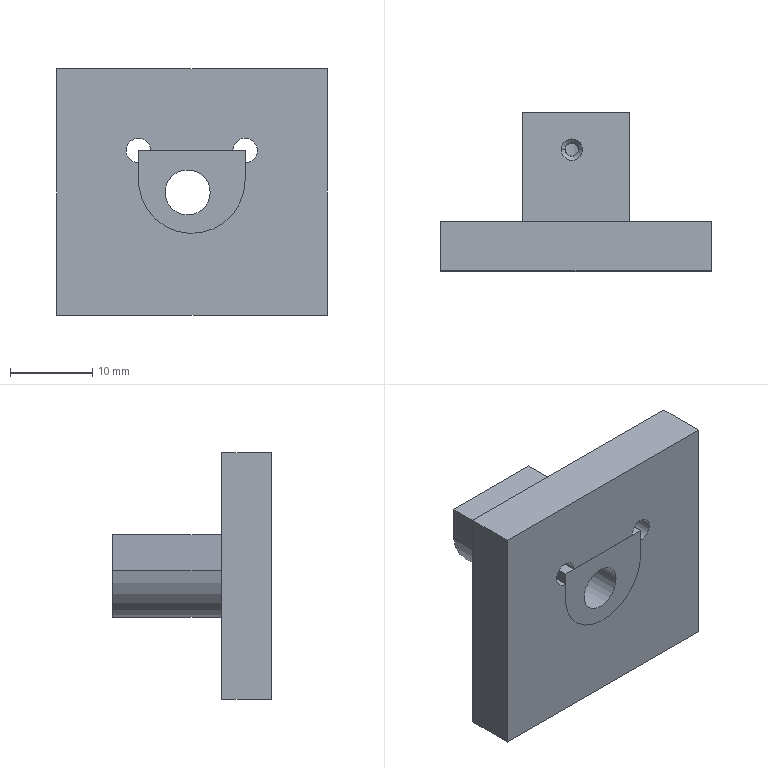NC program | NX | posted with a generic post | part box 32.951 x 19.3 x 30.1 mm
Lines 1 to 1088 of 2936:
N10 G17 G21 G94 G90
(PLANAR_MILL_1 , TOOL : D2)
N12 T02 M6
N14 G54
N16 G17 G0 G90 X0.034 Y0.295 B0. C0. S9500 M3
N18 G43 Z30. H2
N20 Z0.5
N22 G94 G1 X-0.05 Y0.514 Z0.492 F1200.
N24 Y-0.563 Z0.454
N26 X0.058 Y-0.281 Z0.444
N28 Y0.233 Z0.426
N30 X-0.05 Y0.514 Z0.415
N32 Y-0.563 Z0.378
N34 X0.058 Y-0.281 Z0.367
N36 Y0.233 Z0.349
N38 X-0.05 Y0.514 Z0.339
N40 Y-0.563 Z0.301
N42 X0.058 Y-0.281 Z0.29
N44 Y0.233 Z0.272
N46 X-0.05 Y0.514 Z0.262
N48 Y-0.563 Z0.224
N50 X0.058 Y-0.281 Z0.214
N52 Y0.233 Z0.196
N54 X-0.05 Y0.514 Z0.185
N56 Y-0.563 Z0.148
N58 X0.058 Y-0.281 Z0.137
N60 Y0.233 Z0.119
N62 X-0.05 Y0.514 Z0.109
N64 Y-0.563 Z0.071
N66 X0.058 Y-0.281 Z0.061
N68 Y0.233 Z0.043
N70 X-0.05 Y0.514 Z0.032
N72 Y-0.563 Z-0.006
N74 X0.058 Y-0.281 Z-0.016
N76 Y0.233 Z-0.034
N78 X-0.05 Y0.514 Z-0.045
N80 Y-0.563 Z-0.082
N82 X0.058 Y-0.281 Z-0.093
N84 Y0.233 Z-0.111
N86 X-0.05 Y0.514 Z-0.121
N88 Y-0.024 Z-0.14
N90 Y-0.563
N92 G3 X-0.05 Y0.514 R1.5
N94 G1 Y-0.024
N96 X-1.05
N98 Y-2.48
N100 X-0.976 Y-2.479
N102 G3 X-1.05 Y2.443 R2.5
N104 G1 Y-0.024
N106 X-2.05
N108 Y-3.491
N110 X-0.882 Y-3.478
N112 G3 X-1.45 Y3.476 R3.5
N114 G1 X-2.05
N116 Y-0.024
N118 X-3.05
N120 Y-4.502
N122 X-0.799 Y-4.477
N124 G3 X-1.45 Y4.476 R4.5
N126 G1 X-3.05
N128 Y-0.024
N130 X-4.05
N132 Y-5.024
N134 G2 X-5.05 Y-6.024 R1.
N136 G3 X-4.55 Y-6.519 R-0.5
N138 G2 X-3.561 Y-5.508 R1.
N140 G1 X-0.725 Y-5.476
N142 G3 X-1.45 Y5.476 R5.5
N144 G1 X-3.55
N146 G2 X-4.55 Y6.476 R1.
N148 G3 X-5.05 Y5.976 R-0.5
N150 G2 X-4.05 Y4.976 R1.
N152 G1 Y-0.024
N154 Z0.36
N156 G0 X0.034 Y0.295
N158 G1 X-0.05 Y0.514 Z0.352
N160 Y-0.563 Z0.314
N162 X0.058 Y-0.281 Z0.304
N164 Y0.233 Z0.286
N166 X-0.05 Y0.514 Z0.275
N168 Y-0.563 Z0.238
N170 X0.058 Y-0.281 Z0.227
N172 Y0.233 Z0.209
N174 X-0.05 Y0.514 Z0.199
N176 Y-0.563 Z0.161
N178 X0.058 Y-0.281 Z0.15
N180 Y0.233 Z0.132
N182 X-0.05 Y0.514 Z0.122
N184 Y-0.563 Z0.084
N186 X0.058 Y-0.281 Z0.074
N188 Y0.233 Z0.056
N190 X-0.05 Y0.514 Z0.045
N192 Y-0.563 Z0.008
N194 X0.058 Y-0.281 Z-0.003
N196 Y0.233 Z-0.021
N198 X-0.05 Y0.514 Z-0.031
N200 Y-0.563 Z-0.069
N202 X0.058 Y-0.281 Z-0.079
N204 Y0.233 Z-0.097
N206 X-0.05 Y0.514 Z-0.108
N208 Y-0.563 Z-0.146
N210 X0.058 Y-0.281 Z-0.156
N212 Y0.233 Z-0.174
N214 X-0.05 Y0.514 Z-0.185
N216 Y-0.563 Z-0.222
N218 X0.058 Y-0.281 Z-0.233
N220 Y0.233 Z-0.251
N222 X-0.05 Y0.514 Z-0.261
N224 Y-0.024 Z-0.28
N226 Y-0.563
N228 G3 X-0.05 Y0.514 R1.5
N230 G1 Y-0.024
N232 X-1.05
N234 Y-2.48
N236 X-0.976 Y-2.479
N238 G3 X-1.05 Y2.443 R2.5
N240 G1 Y-0.024
N242 X-2.05
N244 Y-3.491
N246 X-0.882 Y-3.478
N248 G3 X-1.45 Y3.476 R3.5
N250 G1 X-2.05
N252 Y-0.024
N254 X-3.05
N256 Y-4.502
N258 X-0.799 Y-4.477
N260 G3 X-1.45 Y4.476 R4.5
N262 G1 X-3.05
N264 Y-0.024
N266 X-4.05
N268 Y-5.024
N270 G2 X-5.05 Y-6.024 R1.
N272 G3 X-4.55 Y-6.519 R-0.5
N274 G2 X-3.561 Y-5.508 R1.
N276 G1 X-0.725 Y-5.476
N278 G3 X-1.45 Y5.476 R5.5
N280 G1 X-3.55
N282 G2 X-4.55 Y6.476 R1.
N284 G3 X-5.05 Y5.976 R-0.5
N286 G2 X-4.05 Y4.976 R1.
N288 G1 Y-0.024
N290 Z0.22
N292 G0 X0.034 Y0.295
N294 G1 X-0.05 Y0.514 Z0.212
N296 Y-0.563 Z0.174
N298 X0.058 Y-0.281 Z0.164
N300 Y0.233 Z0.146
N302 X-0.05 Y0.514 Z0.135
N304 Y-0.563 Z0.098
N306 X0.058 Y-0.281 Z0.087
N308 Y0.233 Z0.069
N310 X-0.05 Y0.514 Z0.059
N312 Y-0.563 Z0.021
N314 X0.058 Y-0.281 Z0.01
N316 Y0.233 Z-0.008
N318 X-0.05 Y0.514 Z-0.018
N320 Y-0.563 Z-0.056
N322 X0.058 Y-0.281 Z-0.066
N324 Y0.233 Z-0.084
N326 X-0.05 Y0.514 Z-0.095
N328 Y-0.563 Z-0.132
N330 X0.058 Y-0.281 Z-0.143
N332 Y0.233 Z-0.161
N334 X-0.05 Y0.514 Z-0.171
N336 Y-0.563 Z-0.209
N338 X0.058 Y-0.281 Z-0.219
N340 Y0.233 Z-0.237
N342 X-0.05 Y0.514 Z-0.248
N344 Y-0.563 Z-0.286
N346 X0.058 Y-0.281 Z-0.296
N348 Y0.233 Z-0.314
N350 X-0.05 Y0.514 Z-0.325
N352 Y-0.563 Z-0.362
N354 X0.058 Y-0.281 Z-0.373
N356 Y0.233 Z-0.391
N358 X-0.05 Y0.514 Z-0.401
N360 Y-0.024 Z-0.42
N362 Y-0.563
N364 G3 X-0.05 Y0.514 R1.5
N366 G1 Y-0.024
N368 X-1.05
N370 Y-2.48
N372 X-0.976 Y-2.479
N374 G3 X-1.05 Y2.443 R2.5
N376 G1 Y-0.024
N378 X-2.05
N380 Y-3.491
N382 X-0.882 Y-3.478
N384 G3 X-1.45 Y3.476 R3.5
N386 G1 X-2.05
N388 Y-0.024
N390 X-3.05
N392 Y-4.502
N394 X-0.799 Y-4.477
N396 G3 X-1.45 Y4.476 R4.5
N398 G1 X-3.05
N400 Y-0.024
N402 X-4.05
N404 Y-5.024
N406 G2 X-5.05 Y-6.024 R1.
N408 G3 X-4.55 Y-6.519 R-0.5
N410 G2 X-3.561 Y-5.508 R1.
N412 G1 X-0.725 Y-5.476
N414 G3 X-1.45 Y5.476 R5.5
N416 G1 X-3.55
N418 G2 X-4.55 Y6.476 R1.
N420 G3 X-5.05 Y5.976 R-0.5
N422 G2 X-4.05 Y4.976 R1.
N424 G1 Y-0.024
N426 Z0.08
N428 G0 X0.034 Y0.295
N430 G1 X-0.05 Y0.514 Z0.072
N432 Y-0.563 Z0.034
N434 X0.058 Y-0.281 Z0.024
N436 Y0.233 Z0.006
N438 X-0.05 Y0.514 Z-0.005
N440 Y-0.563 Z-0.042
N442 X0.058 Y-0.281 Z-0.053
N444 Y0.233 Z-0.071
N446 X-0.05 Y0.514 Z-0.081
N448 Y-0.563 Z-0.119
N450 X0.058 Y-0.281 Z-0.13
N452 Y0.233 Z-0.148
N454 X-0.05 Y0.514 Z-0.158
N456 Y-0.563 Z-0.196
N458 X0.058 Y-0.281 Z-0.206
N460 Y0.233 Z-0.224
N462 X-0.05 Y0.514 Z-0.235
N464 Y-0.563 Z-0.272
N466 X0.058 Y-0.281 Z-0.283
N468 Y0.233 Z-0.301
N470 X-0.05 Y0.514 Z-0.311
N472 Y-0.563 Z-0.349
N474 X0.058 Y-0.281 Z-0.359
N476 Y0.233 Z-0.377
N478 X-0.05 Y0.514 Z-0.388
N480 Y-0.563 Z-0.426
N482 X0.058 Y-0.281 Z-0.436
N484 Y0.233 Z-0.454
N486 X-0.05 Y0.514 Z-0.465
N488 Y-0.563 Z-0.502
N490 X0.058 Y-0.281 Z-0.513
N492 Y0.233 Z-0.531
N494 X-0.05 Y0.514 Z-0.541
N496 Y-0.024 Z-0.56
N498 Y-0.563
N500 G3 X-0.05 Y0.514 R1.5
N502 G1 Y-0.024
N504 X-1.05
N506 Y-2.48
N508 X-0.976 Y-2.479
N510 G3 X-1.05 Y2.443 R2.5
N512 G1 Y-0.024
N514 X-2.05
N516 Y-3.491
N518 X-0.882 Y-3.478
N520 G3 X-1.45 Y3.476 R3.5
N522 G1 X-2.05
N524 Y-0.024
N526 X-3.05
N528 Y-4.502
N530 X-0.799 Y-4.477
N532 G3 X-1.45 Y4.476 R4.5
N534 G1 X-3.05
N536 Y-0.024
N538 X-4.05
N540 Y-5.024
N542 G2 X-5.05 Y-6.024 R1.
N544 G3 X-4.55 Y-6.519 R-0.5
N546 G2 X-3.561 Y-5.508 R1.
N548 G1 X-0.725 Y-5.476
N550 G3 X-1.45 Y5.476 R5.5
N552 G1 X-3.55
N554 G2 X-4.55 Y6.476 R1.
N556 G3 X-5.05 Y5.976 R-0.5
N558 G2 X-4.05 Y4.976 R1.
N560 G1 Y-0.024
N562 Z-0.06
N564 G0 X0.034 Y0.295
N566 G1 X-0.05 Y0.514 Z-0.068
N568 Y-0.563 Z-0.106
N570 X0.058 Y-0.281 Z-0.116
N572 Y0.233 Z-0.134
N574 X-0.05 Y0.514 Z-0.145
N576 Y-0.563 Z-0.182
N578 X0.058 Y-0.281 Z-0.193
N580 Y0.233 Z-0.211
N582 X-0.05 Y0.514 Z-0.221
N584 Y-0.563 Z-0.259
N586 X0.058 Y-0.281 Z-0.27
N588 Y0.233 Z-0.288
N590 X-0.05 Y0.514 Z-0.298
N592 Y-0.563 Z-0.336
N594 X0.058 Y-0.281 Z-0.346
N596 Y0.233 Z-0.364
N598 X-0.05 Y0.514 Z-0.375
N600 Y-0.563 Z-0.412
N602 X0.058 Y-0.281 Z-0.423
N604 Y0.233 Z-0.441
N606 X-0.05 Y0.514 Z-0.451
N608 Y-0.563 Z-0.489
N610 X0.058 Y-0.281 Z-0.499
N612 Y0.233 Z-0.517
N614 X-0.05 Y0.514 Z-0.528
N616 Y-0.563 Z-0.566
N618 X0.058 Y-0.281 Z-0.576
N620 Y0.233 Z-0.594
N622 X-0.05 Y0.514 Z-0.605
N624 Y-0.563 Z-0.642
N626 X0.058 Y-0.281 Z-0.653
N628 Y0.233 Z-0.671
N630 X-0.05 Y0.514 Z-0.681
N632 Y-0.024 Z-0.7
N634 Y-0.563
N636 G3 X-0.05 Y0.514 R1.5
N638 G1 Y-0.024
N640 X-1.05
N642 Y-2.48
N644 X-0.976 Y-2.479
N646 G3 X-1.05 Y2.443 R2.5
N648 G1 Y-0.024
N650 X-2.05
N652 Y-3.491
N654 X-0.882 Y-3.478
N656 G3 X-1.45 Y3.476 R3.5
N658 G1 X-2.05
N660 Y-0.024
N662 X-3.05
N664 Y-4.502
N666 X-0.799 Y-4.477
N668 G3 X-1.45 Y4.476 R4.5
N670 G1 X-3.05
N672 Y-0.024
N674 X-4.05
N676 Y-5.024
N678 G2 X-5.05 Y-6.024 R1.
N680 G3 X-4.55 Y-6.519 R-0.5
N682 G2 X-3.561 Y-5.508 R1.
N684 G1 X-0.725 Y-5.476
N686 G3 X-1.45 Y5.476 R5.5
N688 G1 X-3.55
N690 G2 X-4.55 Y6.476 R1.
N692 G3 X-5.05 Y5.976 R-0.5
N694 G2 X-4.05 Y4.976 R1.
N696 G1 Y-0.024
N698 Z-0.2
N700 G0 X0.034 Y0.295
N702 G1 X-0.05 Y0.514 Z-0.208
N704 Y-0.563 Z-0.246
N706 X0.058 Y-0.281 Z-0.256
N708 Y0.233 Z-0.274
N710 X-0.05 Y0.514 Z-0.285
N712 Y-0.563 Z-0.322
N714 X0.058 Y-0.281 Z-0.333
N716 Y0.233 Z-0.351
N718 X-0.05 Y0.514 Z-0.361
N720 Y-0.563 Z-0.399
N722 X0.058 Y-0.281 Z-0.41
N724 Y0.233 Z-0.428
N726 X-0.05 Y0.514 Z-0.438
N728 Y-0.563 Z-0.476
N730 X0.058 Y-0.281 Z-0.486
N732 Y0.233 Z-0.504
N734 X-0.05 Y0.514 Z-0.515
N736 Y-0.563 Z-0.552
N738 X0.058 Y-0.281 Z-0.563
N740 Y0.233 Z-0.581
N742 X-0.05 Y0.514 Z-0.591
N744 Y-0.563 Z-0.629
N746 X0.058 Y-0.281 Z-0.639
N748 Y0.233 Z-0.657
N750 X-0.05 Y0.514 Z-0.668
N752 Y-0.563 Z-0.706
N754 X0.058 Y-0.281 Z-0.716
N756 Y0.233 Z-0.734
N758 X-0.05 Y0.514 Z-0.745
N760 Y-0.563 Z-0.782
N762 X0.058 Y-0.281 Z-0.793
N764 Y0.233 Z-0.811
N766 X-0.05 Y0.514 Z-0.821
N768 Y-0.024 Z-0.84
N770 Y-0.563
N772 G3 X-0.05 Y0.514 R1.5
N774 G1 Y-0.024
N776 X-1.05
N778 Y-2.48
N780 X-0.976 Y-2.479
N782 G3 X-1.05 Y2.443 R2.5
N784 G1 Y-0.024
N786 X-2.05
N788 Y-3.491
N790 X-0.882 Y-3.478
N792 G3 X-1.45 Y3.476 R3.5
N794 G1 X-2.05
N796 Y-0.024
N798 X-3.05
N800 Y-4.502
N802 X-0.799 Y-4.477
N804 G3 X-1.45 Y4.476 R4.5
N806 G1 X-3.05
N808 Y-0.024
N810 X-4.05
N812 Y-5.024
N814 G2 X-5.05 Y-6.024 R1.
N816 G3 X-4.55 Y-6.519 R-0.5
N818 G2 X-3.561 Y-5.508 R1.
N820 G1 X-0.725 Y-5.476
N822 G3 X-1.45 Y5.476 R5.5
N824 G1 X-3.55
N826 G2 X-4.55 Y6.476 R1.
N828 G3 X-5.05 Y5.976 R-0.5
N830 G2 X-4.05 Y4.976 R1.
N832 G1 Y-0.024
N834 Z-0.34
N836 G0 X0.034 Y0.295
N838 G1 X-0.05 Y0.514 Z-0.348
N840 Y-0.563 Z-0.386
N842 X0.058 Y-0.281 Z-0.396
N844 Y0.233 Z-0.414
N846 X-0.05 Y0.514 Z-0.425
N848 Y-0.563 Z-0.462
N850 X0.058 Y-0.281 Z-0.473
N852 Y0.233 Z-0.491
N854 X-0.05 Y0.514 Z-0.501
N856 Y-0.563 Z-0.539
N858 X0.058 Y-0.281 Z-0.55
N860 Y0.233 Z-0.568
N862 X-0.05 Y0.514 Z-0.578
N864 Y-0.563 Z-0.616
N866 X0.058 Y-0.281 Z-0.626
N868 Y0.233 Z-0.644
N870 X-0.05 Y0.514 Z-0.655
N872 Y-0.563 Z-0.692
N874 X0.058 Y-0.281 Z-0.703
N876 Y0.233 Z-0.721
N878 X-0.05 Y0.514 Z-0.731
N880 Y-0.563 Z-0.769
N882 X0.058 Y-0.281 Z-0.779
N884 Y0.233 Z-0.797
N886 X-0.05 Y0.514 Z-0.808
N888 Y-0.563 Z-0.846
N890 X0.058 Y-0.281 Z-0.856
N892 Y0.233 Z-0.874
N894 X-0.05 Y0.514 Z-0.885
N896 Y-0.563 Z-0.922
N898 X0.058 Y-0.281 Z-0.933
N900 Y0.233 Z-0.951
N902 X-0.05 Y0.514 Z-0.961
N904 Y-0.024 Z-0.98
N906 Y-0.563
N908 G3 X-0.05 Y0.514 R1.5
N910 G1 Y-0.024
N912 X-1.05
N914 Y-2.48
N916 X-0.976 Y-2.479
N918 G3 X-1.05 Y2.443 R2.5
N920 G1 Y-0.024
N922 X-2.05
N924 Y-3.491
N926 X-0.882 Y-3.478
N928 G3 X-1.45 Y3.476 R3.5
N930 G1 X-2.05
N932 Y-0.024
N934 X-3.05
N936 Y-4.502
N938 X-0.799 Y-4.477
N940 G3 X-1.45 Y4.476 R4.5
N942 G1 X-3.05
N944 Y-0.024
N946 X-4.05
N948 Y-5.024
N950 G2 X-5.05 Y-6.024 R1.
N952 G3 X-4.55 Y-6.519 R-0.5
N954 G2 X-3.561 Y-5.508 R1.
N956 G1 X-0.725 Y-5.476
N958 G3 X-1.45 Y5.476 R5.5
N960 G1 X-3.55
N962 G2 X-4.55 Y6.476 R1.
N964 G3 X-5.05 Y5.976 R-0.5
N966 G2 X-4.05 Y4.976 R1.
N968 G1 Y-0.024
N970 Z-0.48
N972 G0 X0.034 Y0.295
N974 G1 X-0.05 Y0.514 Z-0.488
N976 Y-0.563 Z-0.526
N978 X0.058 Y-0.281 Z-0.536
N980 Y0.233 Z-0.554
N982 X-0.05 Y0.514 Z-0.565
N984 Y-0.563 Z-0.602
N986 X0.058 Y-0.281 Z-0.613
N988 Y0.233 Z-0.631
N990 X-0.05 Y0.514 Z-0.641
N992 Y-0.563 Z-0.679
N994 X0.058 Y-0.281 Z-0.69
N996 Y0.233 Z-0.708
N998 X-0.05 Y0.514 Z-0.718
N1000 Y-0.563 Z-0.756
N1002 X0.058 Y-0.281 Z-0.766
N1004 Y0.233 Z-0.784
N1006 X-0.05 Y0.514 Z-0.795
N1008 Y-0.563 Z-0.832
N1010 X0.058 Y-0.281 Z-0.843
N1012 Y0.233 Z-0.861
N1014 X-0.05 Y0.514 Z-0.871
N1016 Y-0.563 Z-0.909
N1018 X0.058 Y-0.281 Z-0.919
N1020 Y0.233 Z-0.937
N1022 X-0.05 Y0.514 Z-0.948
N1024 Y-0.563 Z-0.986
N1026 X0.058 Y-0.281 Z-0.996
N1028 Y0.233 Z-1.014
N1030 X-0.05 Y0.514 Z-1.025
N1032 Y-0.563 Z-1.062
N1034 X0.058 Y-0.281 Z-1.073
N1036 Y0.233 Z-1.091
N1038 X-0.05 Y0.514 Z-1.101
N1040 Y-0.024 Z-1.12
N1042 Y-0.563
N1044 G3 X-0.05 Y0.514 R1.5
N1046 G1 Y-0.024
N1048 X-1.05
N1050 Y-2.48
N1052 X-0.976 Y-2.479
N1054 G3 X-1.05 Y2.443 R2.5
N1056 G1 Y-0.024
N1058 X-2.05
N1060 Y-3.491
N1062 X-0.882 Y-3.478
N1064 G3 X-1.45 Y3.476 R3.5
N1066 G1 X-2.05
N1068 Y-0.024
N1070 X-3.05
N1072 Y-4.502
N1074 X-0.799 Y-4.477
N1076 G3 X-1.45 Y4.476 R4.5
N1078 G1 X-3.05
N1080 Y-0.024
N1082 X-4.05
N1084 Y-5.024
N1086 G2 X-5.05 Y-6.024 R1.
N1088 G3 X-4.55 Y-6.519 R-0.5
N1090 G2 X-3.561 Y-5.508 R1.
N1092 G1 X-0.725 Y-5.476
N1094 G3 X-1.45 Y5.476 R5.5
N1096 G1 X-3.55
N1098 G2 X-4.55 Y6.476 R1.
N1100 G3 X-5.05 Y5.976 R-0.5
N1102 G2 X-4.05 Y4.976 R1.
N1104 G1 Y-0.024
N1106 Z-0.62
N1108 G0 X0.034 Y0.295
N1110 G1 X-0.05 Y0.514 Z-0.628
N1112 Y-0.563 Z-0.666
N1114 X0.058 Y-0.281 Z-0.676
N1116 Y0.233 Z-0.694
N1118 X-0.05 Y0.514 Z-0.705
N1120 Y-0.563 Z-0.742
N1122 X0.058 Y-0.281 Z-0.753
N1124 Y0.233 Z-0.771
N1126 X-0.05 Y0.514 Z-0.781
N1128 Y-0.563 Z-0.819
N1130 X0.058 Y-0.281 Z-0.83
N1132 Y0.233 Z-0.848
N1134 X-0.05 Y0.514 Z-0.858
N1136 Y-0.563 Z-0.896
N1138 X0.058 Y-0.281 Z-0.906
N1140 Y0.233 Z-0.924
N1142 X-0.05 Y0.514 Z-0.935
N1144 Y-0.563 Z-0.972
N1146 X0.058 Y-0.281 Z-0.983
N1148 Y0.233 Z-1.001
N1150 X-0.05 Y0.514 Z-1.011
N1152 Y-0.563 Z-1.049
N1154 X0.058 Y-0.281 Z-1.059
N1156 Y0.233 Z-1.077
N1158 X-0.05 Y0.514 Z-1.088
N1160 Y-0.563 Z-1.126
N1162 X0.058 Y-0.281 Z-1.136
N1164 Y0.233 Z-1.154
N1166 X-0.05 Y0.514 Z-1.165
N1168 Y-0.563 Z-1.202
N1170 X0.058 Y-0.281 Z-1.213
N1172 Y0.233 Z-1.231
N1174 X-0.05 Y0.514 Z-1.241
N1176 Y-0.024 Z-1.26
N1178 Y-0.563
N1180 G3 X-0.05 Y0.514 R1.5
N1182 G1 Y-0.024
N1184 X-1.05
N1186 Y-2.48
N1188 X-0.976 Y-2.479
N1190 G3 X-1.05 Y2.443 R2.5
N1192 G1 Y-0.024
N1194 X-2.05
N1196 Y-3.491
N1198 X-0.882 Y-3.478
N1200 G3 X-1.45 Y3.476 R3.5
N1202 G1 X-2.05
N1204 Y-0.024
N1206 X-3.05
N1208 Y-4.502
N1210 X-0.799 Y-4.477
N1212 G3 X-1.45 Y4.476 R4.5
N1214 G1 X-3.05
N1216 Y-0.024
N1218 X-4.05
N1220 Y-5.024
N1222 G2 X-5.05 Y-6.024 R1.
N1224 G3 X-4.55 Y-6.519 R-0.5
N1226 G2 X-3.561 Y-5.508 R1.
N1228 G1 X-0.725 Y-5.476
N1230 G3 X-1.45 Y5.476 R5.5
N1232 G1 X-3.55
N1234 G2 X-4.55 Y6.476 R1.
N1236 G3 X-5.05 Y5.976 R-0.5
N1238 G2 X-4.05 Y4.976 R1.
N1240 G1 Y-0.024
N1242 Z-0.76
N1244 G0 X0.034 Y0.295
N1246 G1 X-0.05 Y0.514 Z-0.768
N1248 Y-0.563 Z-0.806
N1250 X0.058 Y-0.281 Z-0.816
N1252 Y0.233 Z-0.834
N1254 X-0.05 Y0.514 Z-0.845
N1256 Y-0.563 Z-0.882
N1258 X0.058 Y-0.281 Z-0.893
N1260 Y0.233 Z-0.911
N1262 X-0.05 Y0.514 Z-0.921
N1264 Y-0.563 Z-0.959
N1266 X0.058 Y-0.281 Z-0.97
N1268 Y0.233 Z-0.988
N1270 X-0.05 Y0.514 Z-0.998
N1272 Y-0.563 Z-1.036
N1274 X0.058 Y-0.281 Z-1.046
N1276 Y0.233 Z-1.064
N1278 X-0.05 Y0.514 Z-1.075
N1280 Y-0.563 Z-1.112
N1282 X0.058 Y-0.281 Z-1.123
N1284 Y0.233 Z-1.141
N1286 X-0.05 Y0.514 Z-1.151
N1288 Y-0.563 Z-1.189
N1290 X0.058 Y-0.281 Z-1.199
N1292 Y0.233 Z-1.217
N1294 X-0.05 Y0.514 Z-1.228
N1296 Y-0.563 Z-1.266
N1298 X0.058 Y-0.281 Z-1.276
N1300 Y0.233 Z-1.294
N1302 X-0.05 Y0.514 Z-1.305
N1304 Y-0.563 Z-1.342
N1306 X0.058 Y-0.281 Z-1.353
N1308 Y0.233 Z-1.371
N1310 X-0.05 Y0.514 Z-1.381
N1312 Y-0.024 Z-1.4
N1314 Y-0.563
N1316 G3 X-0.05 Y0.514 R1.5
N1318 G1 Y-0.024
N1320 X-1.05
N1322 Y-2.48
N1324 X-0.976 Y-2.479
N1326 G3 X-1.05 Y2.443 R2.5
N1328 G1 Y-0.024
N1330 X-2.05
N1332 Y-3.491
N1334 X-0.882 Y-3.478
N1336 G3 X-1.45 Y3.476 R3.5
N1338 G1 X-2.05
N1340 Y-0.024
N1342 X-3.05
N1344 Y-4.502
N1346 X-0.799 Y-4.477
N1348 G3 X-1.45 Y4.476 R4.5
N1350 G1 X-3.05
N1352 Y-0.024
N1354 X-4.05
N1356 Y-5.024
N1358 G2 X-5.05 Y-6.024 R1.
N1360 G3 X-4.55 Y-6.519 R-0.5
N1362 G2 X-3.561 Y-5.508 R1.
N1364 G1 X-0.725 Y-5.476
N1366 G3 X-1.45 Y5.476 R5.5
N1368 G1 X-3.55
N1370 G2 X-4.55 Y6.476 R1.
N1372 G3 X-5.05 Y5.976 R-0.5
N1374 G2 X-4.05 Y4.976 R1.
N1376 G1 Y-0.024
N1378 Z-0.9
N1380 G0 X0.034 Y0.295
N1382 G1 X-0.05 Y0.514 Z-0.908
N1384 Y-0.563 Z-0.946
N1386 X0.058 Y-0.281 Z-0.956
N1388 Y0.233 Z-0.974
N1390 X-0.05 Y0.514 Z-0.985
N1392 Y-0.563 Z-1.022
N1394 X0.058 Y-0.281 Z-1.033
N1396 Y0.233 Z-1.051
N1398 X-0.05 Y0.514 Z-1.061
N1400 Y-0.563 Z-1.099
N1402 X0.058 Y-0.281 Z-1.11
N1404 Y0.233 Z-1.128
N1406 X-0.05 Y0.514 Z-1.138
N1408 Y-0.563 Z-1.176
N1410 X0.058 Y-0.281 Z-1.186
N1412 Y0.233 Z-1.204
N1414 X-0.05 Y0.514 Z-1.215
N1416 Y-0.563 Z-1.252
N1418 X0.058 Y-0.281 Z-1.263
N1420 Y0.233 Z-1.281
N1422 X-0.05 Y0.514 Z-1.291
N1424 Y-0.563 Z-1.329
N1426 X0.058 Y-0.281 Z-1.339
N1428 Y0.233 Z-1.357
N1430 X-0.05 Y0.514 Z-1.368
N1432 Y-0.563 Z-1.406
N1434 X0.058 Y-0.281 Z-1.416
N1436 Y0.233 Z-1.434
N1438 X-0.05 Y0.514 Z-1.445
N1440 Y-0.563 Z-1.482
N1442 X0.058 Y-0.281 Z-1.493
N1444 Y0.233 Z-1.511
N1446 X-0.05 Y0.514 Z-1.521
N1448 Y-0.024 Z-1.54
N1450 Y-0.563
N1452 G3 X-0.05 Y0.514 R1.5
N1454 G1 Y-0.024
N1456 X-1.05
N1458 Y-2.48
N1460 X-0.976 Y-2.479
N1462 G3 X-1.05 Y2.443 R2.5
N1464 G1 Y-0.024
N1466 X-2.05
N1468 Y-3.491
N1470 X-0.882 Y-3.478
N1472 G3 X-1.45 Y3.476 R3.5
N1474 G1 X-2.05
N1476 Y-0.024
N1478 X-3.05
N1480 Y-4.502
N1482 X-0.799 Y-4.477
N1484 G3 X-1.45 Y4.476 R4.5
N1486 G1 X-3.05
N1488 Y-0.024
N1490 X-4.05
N1492 Y-5.024
N1494 G2 X-5.05 Y-6.024 R1.
N1496 G3 X-4.55 Y-6.519 R-0.5
N1498 G2 X-3.561 Y-5.508 R1.
N1500 G1 X-0.725 Y-5.476
N1502 G3 X-1.45 Y5.476 R5.5
N1504 G1 X-3.55
N1506 G2 X-4.55 Y6.476 R1.
N1508 G3 X-5.05 Y5.976 R-0.5
N1510 G2 X-4.05 Y4.976 R1.
N1512 G1 Y-0.024
N1514 Z-1.04
N1516 G0 X0.034 Y0.295
N1518 G1 X-0.05 Y0.514 Z-1.048
N1520 Y-0.563 Z-1.086
N1522 X0.058 Y-0.281 Z-1.096
N1524 Y0.233 Z-1.114
N1526 X-0.05 Y0.514 Z-1.125
N1528 Y-0.563 Z-1.162
N1530 X0.058 Y-0.281 Z-1.173
N1532 Y0.233 Z-1.191
N1534 X-0.05 Y0.514 Z-1.201
N1536 Y-0.563 Z-1.239
N1538 X0.058 Y-0.281 Z-1.25
N1540 Y0.233 Z-1.268
N1542 X-0.05 Y0.514 Z-1.278
N1544 Y-0.563 Z-1.316
N1546 X0.058 Y-0.281 Z-1.326
N1548 Y0.233 Z-1.344
N1550 X-0.05 Y0.514 Z-1.355
N1552 Y-0.563 Z-1.392
N1554 X0.058 Y-0.281 Z-1.403
N1556 Y0.233 Z-1.421
N1558 X-0.05 Y0.514 Z-1.431
N1560 Y-0.563 Z-1.469
N1562 X0.058 Y-0.281 Z-1.479
N1564 Y0.233 Z-1.497
N1566 X-0.05 Y0.514 Z-1.508
N1568 Y-0.563 Z-1.546
N1570 X0.058 Y-0.281 Z-1.556
N1572 Y0.233 Z-1.574
N1574 X-0.05 Y0.514 Z-1.585
N1576 Y-0.563 Z-1.622
N1578 X0.058 Y-0.281 Z-1.633
N1580 Y0.233 Z-1.651
N1582 X-0.05 Y0.514 Z-1.661
N1584 Y-0.024 Z-1.68
N1586 Y-0.563
N1588 G3 X-0.05 Y0.514 R1.5
N1590 G1 Y-0.024
N1592 X-1.05
N1594 Y-2.48
N1596 X-0.976 Y-2.479
N1598 G3 X-1.05 Y2.443 R2.5
N1600 G1 Y-0.024
N1602 X-2.05
N1604 Y-3.491
N1606 X-0.882 Y-3.478
N1608 G3 X-1.45 Y3.476 R3.5
N1610 G1 X-2.05
N1612 Y-0.024
N1614 X-3.05
N1616 Y-4.502
N1618 X-0.799 Y-4.477
N1620 G3 X-1.45 Y4.476 R4.5
N1622 G1 X-3.05
N1624 Y-0.024
N1626 X-4.05
N1628 Y-5.024
N1630 G2 X-5.05 Y-6.024 R1.
N1632 G3 X-4.55 Y-6.519 R-0.5
N1634 G2 X-3.561 Y-5.508 R1.
N1636 G1 X-0.725 Y-5.476
N1638 G3 X-1.45 Y5.476 R5.5
N1640 G1 X-3.55
N1642 G2 X-4.55 Y6.476 R1.
N1644 G3 X-5.05 Y5.976 R-0.5
N1646 G2 X-4.05 Y4.976 R1.
N1648 G1 Y-0.024
N1650 Z-1.18
N1652 G0 X0.034 Y0.295
N1654 G1 X-0.05 Y0.514 Z-1.188
N1656 Y-0.563 Z-1.226
N1658 X0.058 Y-0.281 Z-1.236
N1660 Y0.233 Z-1.254
N1662 X-0.05 Y0.514 Z-1.265
N1664 Y-0.563 Z-1.302
N1666 X0.058 Y-0.281 Z-1.313
N1668 Y0.233 Z-1.331
N1670 X-0.05 Y0.514 Z-1.341
N1672 Y-0.563 Z-1.379
N1674 X0.058 Y-0.281 Z-1.39
N1676 Y0.233 Z-1.408
N1678 X-0.05 Y0.514 Z-1.418
N1680 Y-0.563 Z-1.456
N1682 X0.058 Y-0.281 Z-1.466
N1684 Y0.233 Z-1.484
N1686 X-0.05 Y0.514 Z-1.495
N1688 Y-0.563 Z-1.532
N1690 X0.058 Y-0.281 Z-1.543
N1692 Y0.233 Z-1.561
N1694 X-0.05 Y0.514 Z-1.571
N1696 Y-0.563 Z-1.609
N1698 X0.058 Y-0.281 Z-1.619
N1700 Y0.233 Z-1.637
N1702 X-0.05 Y0.514 Z-1.648
N1704 Y-0.563 Z-1.686
N1706 X0.058 Y-0.281 Z-1.696
N1708 Y0.233 Z-1.714
N1710 X-0.05 Y0.514 Z-1.725
N1712 Y-0.563 Z-1.762
N1714 X0.058 Y-0.281 Z-1.773
N1716 Y0.233 Z-1.791
N1718 X-0.05 Y0.514 Z-1.801
N1720 Y-0.024 Z-1.82
N1722 Y-0.563
N1724 G3 X-0.05 Y0.514 R1.5
N1726 G1 Y-0.024
N1728 X-1.05
N1730 Y-2.48
N1732 X-0.976 Y-2.479
N1734 G3 X-1.05 Y2.443 R2.5
N1736 G1 Y-0.024
N1738 X-2.05
N1740 Y-3.491
N1742 X-0.882 Y-3.478
N1744 G3 X-1.45 Y3.476 R3.5
N1746 G1 X-2.05
N1748 Y-0.024
N1750 X-3.05
N1752 Y-4.502
N1754 X-0.799 Y-4.477
N1756 G3 X-1.45 Y4.476 R4.5
N1758 G1 X-3.05
N1760 Y-0.024
N1762 X-4.05
N1764 Y-5.024
N1766 G2 X-5.05 Y-6.024 R1.
N1768 G3 X-4.55 Y-6.519 R-0.5
N1770 G2 X-3.561 Y-5.508 R1.
N1772 G1 X-0.725 Y-5.476
N1774 G3 X-1.45 Y5.476 R5.5
N1776 G1 X-3.55
N1778 G2 X-4.55 Y6.476 R1.
N1780 G3 X-5.05 Y5.976 R-0.5
N1782 G2 X-4.05 Y4.976 R1.
N1784 G1 Y-0.024
N1786 Z-1.32
N1788 G0 X0.034 Y0.295
N1790 G1 X-0.05 Y0.514 Z-1.328
N1792 Y-0.563 Z-1.366
N1794 X0.058 Y-0.281 Z-1.376
N1796 Y0.233 Z-1.394
N1798 X-0.05 Y0.514 Z-1.405
N1800 Y-0.563 Z-1.442
N1802 X0.058 Y-0.281 Z-1.453
N1804 Y0.233 Z-1.471
N1806 X-0.05 Y0.514 Z-1.481
N1808 Y-0.563 Z-1.519
N1810 X0.058 Y-0.281 Z-1.53
N1812 Y0.233 Z-1.548
N1814 X-0.05 Y0.514 Z-1.558
N1816 Y-0.563 Z-1.596
N1818 X0.058 Y-0.281 Z-1.606
N1820 Y0.233 Z-1.624
N1822 X-0.05 Y0.514 Z-1.635
N1824 Y-0.563 Z-1.672
N1826 X0.058 Y-0.281 Z-1.683
N1828 Y0.233 Z-1.701
N1830 X-0.05 Y0.514 Z-1.711
N1832 Y-0.563 Z-1.749
N1834 X0.058 Y-0.281 Z-1.759
N1836 Y0.233 Z-1.777
N1838 X-0.05 Y0.514 Z-1.788
N1840 Y-0.563 Z-1.826
N1842 X0.058 Y-0.281 Z-1.836
N1844 Y0.233 Z-1.854
N1846 X-0.05 Y0.514 Z-1.865
N1848 Y-0.563 Z-1.902
N1850 X0.058 Y-0.281 Z-1.913
N1852 Y0.233 Z-1.931
N1854 X-0.05 Y0.514 Z-1.941
N1856 Y-0.024 Z-1.96
N1858 Y-0.563
N1860 G3 X-0.05 Y0.514 R1.5
N1862 G1 Y-0.024
N1864 X-1.05
N1866 Y-2.48
N1868 X-0.976 Y-2.479
N1870 G3 X-1.05 Y2.443 R2.5
N1872 G1 Y-0.024
N1874 X-2.05
N1876 Y-3.491
N1878 X-0.882 Y-3.478
N1880 G3 X-1.45 Y3.476 R3.5
N1882 G1 X-2.05
N1884 Y-0.024
N1886 X-3.05
N1888 Y-4.502
N1890 X-0.799 Y-4.477
N1892 G3 X-1.45 Y4.476 R4.5
N1894 G1 X-3.05
N1896 Y-0.024
N1898 X-4.05
N1900 Y-5.024
N1902 G2 X-5.05 Y-6.024 R1.
N1904 G3 X-4.55 Y-6.519 R-0.5
N1906 G2 X-3.561 Y-5.508 R1.
N1908 G1 X-0.725 Y-5.476
N1910 G3 X-1.45 Y5.476 R5.5
N1912 G1 X-3.55
N1914 G2 X-4.55 Y6.476 R1.
N1916 G3 X-5.05 Y5.976 R-0.5
N1918 G2 X-4.05 Y4.976 R1.
N1920 G1 Y-0.024
N1922 Z-1.46
N1924 G0 X0.034 Y0.295
N1926 G1 X-0.05 Y0.514 Z-1.468
N1928 Y-0.563 Z-1.506
N1930 X0.058 Y-0.281 Z-1.516
N1932 Y0.233 Z-1.534
N1934 X-0.05 Y0.514 Z-1.545
N1936 Y-0.563 Z-1.582
N1938 X0.058 Y-0.281 Z-1.593
N1940 Y0.233 Z-1.611
N1942 X-0.05 Y0.514 Z-1.621
N1944 Y-0.563 Z-1.659
N1946 X0.058 Y-0.281 Z-1.67
N1948 Y0.233 Z-1.688
N1950 X-0.05 Y0.514 Z-1.698
N1952 Y-0.563 Z-1.736
N1954 X0.058 Y-0.281 Z-1.746
N1956 Y0.233 Z-1.764
N1958 X-0.05 Y0.514 Z-1.775
N1960 Y-0.563 Z-1.812
N1962 X0.058 Y-0.281 Z-1.823
N1964 Y0.233 Z-1.841
N1966 X-0.05 Y0.514 Z-1.851
N1968 Y-0.563 Z-1.889
N1970 X0.058 Y-0.281 Z-1.899
N1972 Y0.233 Z-1.917
N1974 X-0.05 Y0.514 Z-1.928
N1976 Y-0.563 Z-1.966
N1978 X0.058 Y-0.281 Z-1.976
N1980 Y0.233 Z-1.994
N1982 X-0.05 Y0.514 Z-2.005
N1984 Y-0.563 Z-2.042
N1986 X0.058 Y-0.281 Z-2.053
N1988 Y0.233 Z-2.071
N1990 X-0.05 Y0.514 Z-2.081
N1992 Y-0.024 Z-2.1
N1994 Y-0.563
N1996 G3 X-0.05 Y0.514 R1.5
N1998 G1 Y-0.024
N2000 X-1.05
N2002 Y-2.48
N2004 X-0.976 Y-2.479
N2006 G3 X-1.05 Y2.443 R2.5
N2008 G1 Y-0.024
N2010 X-2.05
N2012 Y-3.491
N2014 X-0.882 Y-3.478
N2016 G3 X-1.45 Y3.476 R3.5
N2018 G1 X-2.05
N2020 Y-0.024
N2022 X-3.05
N2024 Y-4.502
N2026 X-0.799 Y-4.477
N2028 G3 X-1.45 Y4.476 R4.5
N2030 G1 X-3.05
N2032 Y-0.024
N2034 X-4.05
N2036 Y-5.024
N2038 G2 X-5.05 Y-6.024 R1.
N2040 G3 X-4.55 Y-6.519 R-0.5
N2042 G2 X-3.561 Y-5.508 R1.
N2044 G1 X-0.725 Y-5.476
N2046 G3 X-1.45 Y5.476 R5.5
N2048 G1 X-3.55
N2050 G2 X-4.55 Y6.476 R1.
N2052 G3 X-5.05 Y5.976 R-0.5
N2054 G2 X-4.05 Y4.976 R1.
N2056 G1 Y-0.024
N2058 Z-1.6
N2060 G0 X0.034 Y0.295
N2062 G1 X-0.05 Y0.514 Z-1.608
N2064 Y-0.563 Z-1.646
N2066 X0.058 Y-0.281 Z-1.656
N2068 Y0.233 Z-1.674
N2070 X-0.05 Y0.514 Z-1.685
N2072 Y-0.563 Z-1.722
N2074 X0.058 Y-0.281 Z-1.733
N2076 Y0.233 Z-1.751
N2078 X-0.05 Y0.514 Z-1.761
N2080 Y-0.563 Z-1.799
N2082 X0.058 Y-0.281 Z-1.81
N2084 Y0.233 Z-1.828
N2086 X-0.05 Y0.514 Z-1.838
N2088 Y-0.563 Z-1.876
N2090 X0.058 Y-0.281 Z-1.886
N2092 Y0.233 Z-1.904
N2094 X-0.05 Y0.514 Z-1.915
N2096 Y-0.563 Z-1.952
N2098 X0.058 Y-0.281 Z-1.963
N2100 Y0.233 Z-1.981
N2102 X-0.05 Y0.514 Z-1.991
N2104 Y-0.563 Z-2.029
N2106 X0.058 Y-0.281 Z-2.039
N2108 Y0.233 Z-2.057
N2110 X-0.05 Y0.514 Z-2.068
N2112 Y-0.563 Z-2.106
N2114 X0.058 Y-0.281 Z-2.116
N2116 Y0.233 Z-2.134
N2118 X-0.05 Y0.514 Z-2.145
N2120 Y-0.563 Z-2.182
N2122 X0.058 Y-0.281 Z-2.193
N2124 Y0.233 Z-2.211
N2126 X-0.05 Y0.514 Z-2.221
N2128 Y-0.024 Z-2.24
N2130 Y-0.563
N2132 G3 X-0.05 Y0.514 R1.5
N2134 G1 Y-0.024
N2136 X-1.05
N2138 Y-2.48
N2140 X-0.976 Y-2.479
N2142 G3 X-1.05 Y2.443 R2.5
N2144 G1 Y-0.024
N2146 X-2.05
N2148 Y-3.491
N2150 X-0.882 Y-3.478
N2152 G3 X-1.45 Y3.476 R3.5
N2154 G1 X-2.05
N2156 Y-0.024
N2158 X-3.05
N2160 Y-4.502
N2162 X-0.799 Y-4.477
N2164 G3 X-1.45 Y4.476 R4.5
N2166 G1 X-3.05
N2168 Y-0.024
N2170 X-4.05
N2172 Y-5.024
N2174 G2 X-5.05 Y-6.024 R1.